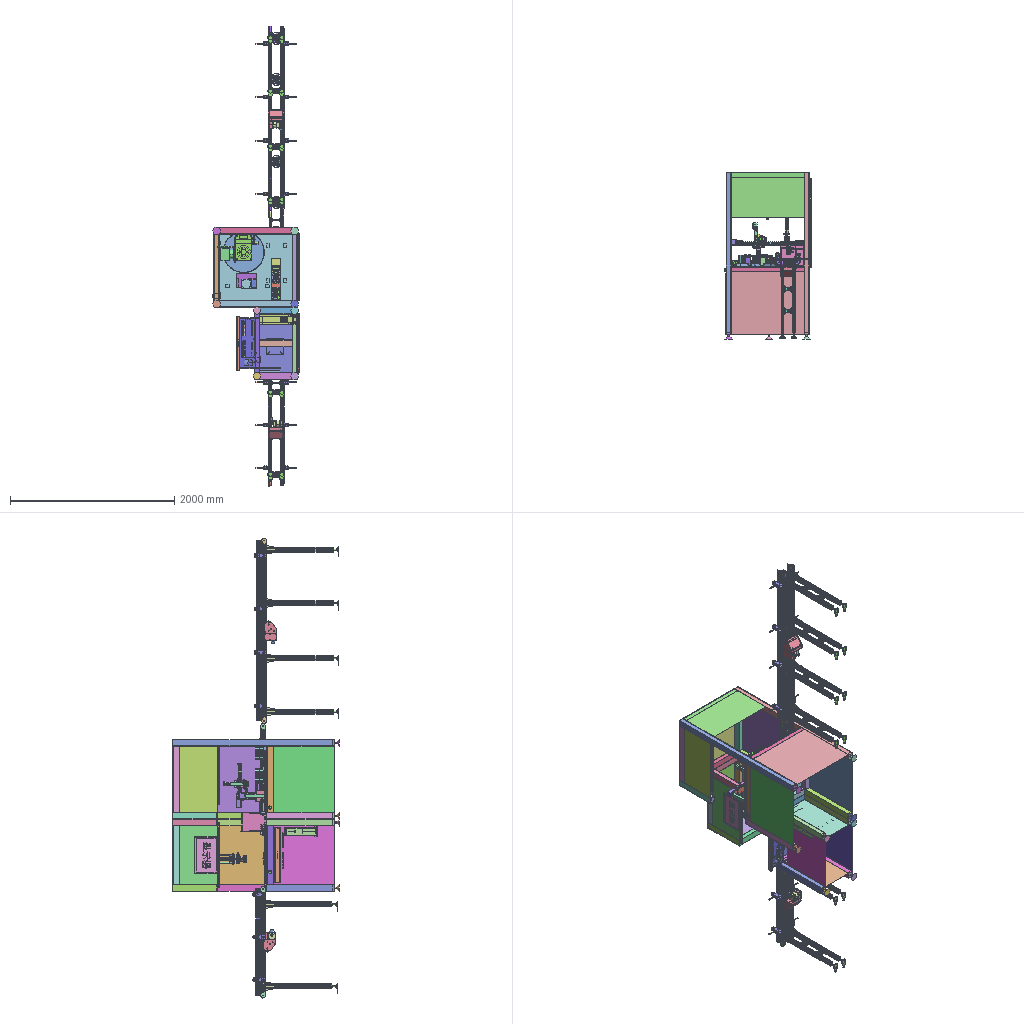Assembly | STEP file | 429 different items | 902 placed | box 1053 x 2031 x 5608 mm
Parts list (item | name | quantity | parent item | size | volume), first 276 of 429 items:
1 | Guide wheel mechanism revised.sldasm-Part-1 (subassembly) | x1 | in 导轮机构Assembly 2 | 80 x 1970 x 60 mm | 1583880 mm3
2 | Guide wheel mechanism revised.sldasm-Part-10 (subassembly) | x1 | in 导轮机构Assembly 2 | 80 x 60 x 890 mm | 715560 mm3
3 | Guide wheel mechanism revised.sldasm-Part-11 (subassembly) | x1 | in 导轮机构Assembly 2 | 972.42 x 1.2 x 1012 mm | 1181397 mm3
4 | Guide wheel mechanism revised.sldasm-Part-12 (subassembly) | x1 | in 导轮机构Assembly 2 | 91.505 x 80 x 91.505 mm | 172572 mm3
5 | Guide wheel mechanism revised.sldasm-Part-13 (subassembly) | x1 | in 导轮机构Assembly 2 | 91.505 x 80 x 91.505 mm | 172572 mm3
6 | Guide wheel mechanism revised.sldasm-Part-14 (subassembly) | x1 | in 导轮机构Assembly 2 | 91.505 x 80 x 91.505 mm | 172572 mm3
7 | Guide wheel mechanism revised.sldasm-Part-145 (subassembly) | x1 | in 导轮机构Assembly 2 | 80 x 1970 x 60 mm | 1583880 mm3
8 | Guide wheel mechanism revised.sldasm-Part-146 (subassembly) | x1 | in 导轮机构Assembly 2 | 80 x 1970 x 60 mm | 1583880 mm3
9 | Guide wheel mechanism revised.sldasm-Part-147 (subassembly) | x1 | in 导轮机构Assembly 2 | 720 x 80 x 60 mm | 578880 mm3
10 | Guide wheel mechanism revised.sldasm-Part-148 (subassembly) | x1 | in 导轮机构Assembly 2 | 720 x 80 x 60 mm | 578880 mm3
11 | Guide wheel mechanism revised.sldasm-Part-149 (subassembly) | x1 | in 导轮机构Assembly 2 | 720 x 80 x 60 mm | 578880 mm3
12 | Guide wheel mechanism revised.sldasm-Part-15 (subassembly) | x1 | in 导轮机构Assembly 2 | 91.505 x 80 x 91.505 mm | 172572 mm3
13 | Guide wheel mechanism revised.sldasm-Part-150 (subassembly) | x1 | in 导轮机构Assembly 2 | 720 x 80 x 60 mm | 578880 mm3
14 | Guide wheel mechanism revised.sldasm-Part-151 (subassembly) | x1 | in 导轮机构Assembly 2 | 80 x 60 x 400 mm | 321600 mm3
15 | Guide wheel mechanism revised.sldasm-Part-152 (subassembly) | x1 | in 导轮机构Assembly 2 | 80 x 60 x 400 mm | 321600 mm3
16 | Guide wheel mechanism revised.sldasm-Part-153 (subassembly) | x1 | in 导轮机构Assembly 2 | 80 x 60 x 400 mm | 321600 mm3
17 | Guide wheel mechanism revised.sldasm-Part-154 (subassembly) | x1 | in 导轮机构Assembly 2 | 80 x 60 x 400 mm | 321600 mm3
18 | Guide wheel mechanism revised.sldasm-Part-155 (subassembly) | x1 | in 导轮机构Assembly 2 | 80 x 60 x 400 mm | 321600 mm3
19 | Guide wheel mechanism revised.sldasm-Part-156 (subassembly) | x1 | in 导轮机构Assembly 2 | 80 x 60 x 400 mm | 321600 mm3
20 | Guide wheel mechanism revised.sldasm-Part-157 (subassembly) | x1 | in 导轮机构Assembly 2 | 882.42 x 8 x 522.42 mm | 3528427 mm3
21 | Guide wheel mechanism revised.sldasm-Part-158 (subassembly) | x1 | in 导轮机构Assembly 2 | 882.42 x 1.2 x 522.42 mm | 553193 mm3
22 | Guide wheel mechanism revised.sldasm-Part-159 (subassembly) | x1 | in 导轮机构Assembly 2 | 91.505 x 80 x 91.505 mm | 172572 mm3
23 | Guide wheel mechanism revised.sldasm-Part-16 (subassembly) | x1 | in 导轮机构Assembly 2 | 25 x 1120 x 25 mm | 195019 mm3
24 | Guide wheel mechanism revised.sldasm-Part-160 (subassembly) | x1 | in 导轮机构Assembly 2 | 91.505 x 80 x 91.505 mm | 172572 mm3
25 | Guide wheel mechanism revised.sldasm-Part-161 (subassembly) | x1 | in 导轮机构Assembly 2 | 91.505 x 80 x 91.505 mm | 172572 mm3
26 | Guide wheel mechanism revised.sldasm-Part-162 (subassembly) | x1 | in 导轮机构Assembly 2 | 91.505 x 80 x 91.505 mm | 172572 mm3
27 | Guide wheel mechanism revised.sldasm-Part-163 (subassembly) | x1 | in 导轮机构Assembly 2 | 25 x 1120 x 25 mm | 195019 mm3
28 | Guide wheel mechanism revised.sldasm-Part-164 (subassembly) | x1 | in 导轮机构Assembly 2 | 770 x 25 x 25 mm | 132103 mm3
29 | Guide wheel mechanism revised.sldasm-Part-165 (subassembly) | x1 | in 导轮机构Assembly 2 | 25 x 1120 x 25 mm | 195019 mm3
30 | Guide wheel mechanism revised.sldasm-Part-166 (subassembly) | x1 | in 导轮机构Assembly 2 | 770 x 25 x 25 mm | 132103 mm3
31 | Guide wheel mechanism revised.sldasm-Part-167 (subassembly) | x1 | in 导轮机构Assembly 2 | 720 x 740 x 2 mm | 886350 mm3
32 | Guide wheel mechanism revised.sldasm-Part-168 (subassembly) | x1 | in 导轮机构Assembly 2 | 1.2 x 760 x 400 mm | 364800 mm3
33 | Guide wheel mechanism revised.sldasm-Part-169 (subassembly) | x1 | in 导轮机构Assembly 2 | 2 x 760 x 403.01 mm | 612575 mm3
34 | Guide wheel mechanism revised.sldasm-Part-17 (subassembly) | x1 | in 导轮机构Assembly 2 | 860 x 25 x 25 mm | 148281 mm3
35 | Guide wheel mechanism revised.sldasm-Part-170 (subassembly) | x1 | in 导轮机构Assembly 2 | 720 x 740 x 1.2 mm | 639360 mm3
36 | Guide wheel mechanism revised.sldasm-Part-171 (subassembly) | x1 | in 导轮机构Assembly 2 | 80 x 828.01 x 60 mm | 665720 mm3
37 | Guide wheel mechanism revised.sldasm-Part-172 (subassembly) | x1 | in 导轮机构Assembly 2 | 80 x 541.99 x 60 mm | 435760 mm3
38 | Guide wheel mechanism revised.sldasm-Part-173 (subassembly) | x1 | in 导轮机构Assembly 2 | 74 x 5 x 54 mm | 19980 mm3
39 | Guide wheel mechanism revised.sldasm-Part-174 (subassembly) | x1 | in 导轮机构Assembly 2 | 74 x 5 x 54 mm | 19980 mm3
40 | Guide wheel mechanism revised.sldasm-Part-175 (subassembly) | x1 | in 导轮机构Assembly 2 | 80 x 60 x 400 mm | 321600 mm3
41 | Guide wheel mechanism revised.sldasm-Part-176 (subassembly) | x1 | in 导轮机构Assembly 2 | 80 x 60 x 400 mm | 217600 mm3
42 | Guide wheel mechanism revised.sldasm-Part-177 (subassembly) | x1 | in 导轮机构Assembly 2 | 720 x 60 x 80 mm | 578880 mm3
43 | Guide wheel mechanism revised.sldasm-Part-178 (subassembly) | x1 | in 导轮机构Assembly 2 | 80 x 828.01 x 60 mm | 665720 mm3
44 | Guide wheel mechanism revised.sldasm-Part-179 (subassembly) | x1 | in 导轮机构Assembly 2 | 80 x 541.99 x 60 mm | 435760 mm3
45 | Guide wheel mechanism revised.sldasm-Part-18 (subassembly) | x1 | in 导轮机构Assembly 2 | 25 x 1120 x 25 mm | 195019 mm3
46 | Guide wheel mechanism revised.sldasm-Part-180 (subassembly) | x1 | in 导轮机构Assembly 2 | 74 x 5 x 54 mm | 19980 mm3
47 | Guide wheel mechanism revised.sldasm-Part-181 (subassembly) | x1 | in 导轮机构Assembly 2 | 74 x 5 x 54 mm | 19980 mm3
48 | Guide wheel mechanism revised.sldasm-Part-182 (subassembly) | x1 | in 导轮机构Assembly 2 | 735 x 1085 x 1.2 mm | 956970 mm3
49 | Guide wheel mechanism revised.sldasm-Part-183 (subassembly) | x1 | in 导轮机构Assembly 2 | 5 x 421.99 x 400 mm | 843980 mm3
50 | Guide wheel mechanism revised.sldasm-Part-184 (subassembly) | x1 | in 导轮机构Assembly 2 | 720 x 461.99 x 3 mm | 633248 mm3
51 | Guide wheel mechanism revised.sldasm-Part-185 (subassembly) | x1 | in 导轮机构Assembly 2 | 22.5 x 75 x 250 mm | 43875 mm3
52 | Guide wheel mechanism revised.sldasm-Part-186 (subassembly) | x1 | in 导轮机构Assembly 2 | 22.5 x 75 x 250 mm | 43875 mm3
53 | Guide wheel mechanism revised.sldasm-Part-187 (subassembly) | x1 | in 导轮机构Assembly 2 | 123 x 31.5 x 458.8 mm | 125941 mm3
54 | Guide wheel mechanism revised.sldasm-Part-188 (subassembly) | x1 | in 导轮机构Assembly 2 | 38 x 275 x 47 mm | 67650 mm3
55 | Guide wheel mechanism revised.sldasm-Part-189 (subassembly) | x1 | in 导轮机构Assembly 2 | 38 x 275 x 45.79 mm | 66652 mm3
56 | Guide wheel mechanism revised.sldasm-Part-19 (subassembly) | x1 | in 导轮机构Assembly 2 | 860 x 25 x 25 mm | 148281 mm3
57 | Guide wheel mechanism revised.sldasm-Part-190 (subassembly) | x1 | in 导轮机构Assembly 2 | 660 x 50 x 30 mm | 98910 mm3
58 | Guide wheel mechanism revised.sldasm-Part-191 (subassembly) | x1 | in 导轮机构Assembly 2 | 600 x 35 x 200 mm | 241391 mm3
59 | Guide wheel mechanism revised.sldasm-Part-192 (subassembly) | x1 | in 导轮机构Assembly 2 | 420.5 x 396 x 106 mm | 15546252 mm3
60 | Guide wheel mechanism revised.sldasm-Part-193 (subassembly) | x2 | in 导轮机构Assembly 2 | 505 x 45 x 12.5 mm | 214790 mm3
61 | Guide wheel mechanism revised.sldasm-Part-194 (subassembly) | x1 | in 导轮机构Assembly 2 | 93.5 x 80 x 103 mm | 26904 mm3
62 | Guide wheel mechanism revised.sldasm-Part-195 (subassembly) | x1 | in 导轮机构Assembly 2 | - | -
63 | Guide wheel mechanism revised.sldasm-Part-196 (subassembly) | x1 | in 导轮机构Assembly 2 | - | -
64 | Guide wheel mechanism revised.sldasm-Part-197 (subassembly) | x1 | in 导轮机构Assembly 2 | - | -
65 | Guide wheel mechanism revised.sldasm-Part-198 (subassembly) | x1 | in 导轮机构Assembly 2 | - | -
66 | Guide wheel mechanism revised.sldasm-Part-199 (subassembly) | x1 | in 导轮机构Assembly 2 | - | -
67 | Guide wheel mechanism revised.sldasm-Part-2 (subassembly) | x1 | in 导轮机构Assembly 2 | 80 x 1970 x 60 mm | 1583880 mm3
68 | Guide wheel mechanism revised.sldasm-Part-20 (subassembly) | x1 | in 导轮机构Assembly 2 | 825 x 1085 x 2 mm | 1790250 mm3
69 | Guide wheel mechanism revised.sldasm-Part-200 (subassembly) | x1 | in 导轮机构Assembly 2 | - | -
70 | Guide wheel mechanism revised.sldasm-Part-201 (subassembly) | x1 | in 导轮机构Assembly 2 | - | -
71 | Guide wheel mechanism revised.sldasm-Part-202 (subassembly) | x1 | in 导轮机构Assembly 2 | - | -
72 | Guide wheel mechanism revised.sldasm-Part-203 (subassembly) | x1 | in 导轮机构Assembly 2 | - | -
73 | Guide wheel mechanism revised.sldasm-Part-204 (subassembly) | x1 | in 导轮机构Assembly 2 | - | -
74 | Guide wheel mechanism revised.sldasm-Part-205 (subassembly) | x1 | in 导轮机构Assembly 2 | - | -
75 | Guide wheel mechanism revised.sldasm-Part-206 (subassembly) | x1 | in 导轮机构Assembly 2 | - | -
76 | Guide wheel mechanism revised.sldasm-Part-207 (subassembly) | x1 | in 导轮机构Assembly 2 | - | -
77 | Guide wheel mechanism revised.sldasm-Part-208 (subassembly) | x1 | in 导轮机构Assembly 2 | - | -
78 | Guide wheel mechanism revised.sldasm-Part-209 (subassembly) | x1 | in 导轮机构Assembly 2 | - | -
79 | Guide wheel mechanism revised.sldasm-Part-21 (subassembly) | x1 | in 导轮机构Assembly 2 | 810 x 740 x 5 mm | 2997000 mm3
80 | Guide wheel mechanism revised.sldasm-Part-210 (subassembly) | x1 | in 导轮机构Assembly 2 | - | -
81 | Guide wheel mechanism revised.sldasm-Part-211 (subassembly) | x1 | in 导轮机构Assembly 2 | - | -
82 | Guide wheel mechanism revised.sldasm-Part-212 (subassembly) | x1 | in 导轮机构Assembly 2 | - | -
83 | Guide wheel mechanism revised.sldasm-Part-213 (subassembly) | x1 | in 导轮机构Assembly 2 | - | -
84 | Guide wheel mechanism revised.sldasm-Part-214 (subassembly) | x1 | in 导轮机构Assembly 2 | - | -
85 | Guide wheel mechanism revised.sldasm-Part-215 (subassembly) | x1 | in 导轮机构Assembly 2 | - | -
86 | Guide wheel mechanism revised.sldasm-Part-216 (subassembly) | x1 | in 导轮机构Assembly 2 | - | -
87 | Guide wheel mechanism revised.sldasm-Part-217 (subassembly) | x1 | in 导轮机构Assembly 2 | - | -
88 | Guide wheel mechanism revised.sldasm-Part-218 (subassembly) | x1 | in 导轮机构Assembly 2 | - | -
89 | Guide wheel mechanism revised.sldasm-Part-219 (subassembly) | x1 | in 导轮机构Assembly 2 | - | -
90 | Guide wheel mechanism revised.sldasm-Part-22 (subassembly) | x1 | in 导轮机构Assembly 2 | 1.2 x 760 x 890 mm | 811680 mm3
91 | Guide wheel mechanism revised.sldasm-Part-220 (subassembly) | x1 | in 导轮机构Assembly 2 | - | -
92 | Guide wheel mechanism revised.sldasm-Part-221 (subassembly) | x1 | in 导轮机构Assembly 2 | - | -
93 | Guide wheel mechanism revised.sldasm-Part-222 (subassembly) | x1 | in 导轮机构Assembly 2 | - | -
94 | Guide wheel mechanism revised.sldasm-Part-223 (subassembly) | x1 | in 导轮机构Assembly 2 | - | -
95 | Guide wheel mechanism revised.sldasm-Part-224 (subassembly) | x1 | in 导轮机构Assembly 2 | - | -
96 | Guide wheel mechanism revised.sldasm-Part-225 (subassembly) | x1 | in 导轮机构Assembly 2 | - | -
97 | Guide wheel mechanism revised.sldasm-Part-226 (subassembly) | x1 | in 导轮机构Assembly 2 | - | -
98 | Guide wheel mechanism revised.sldasm-Part-227 (subassembly) | x1 | in 导轮机构Assembly 2 | - | -
99 | Guide wheel mechanism revised.sldasm-Part-228 (subassembly) | x1 | in 导轮机构Assembly 2 | - | -
100 | Guide wheel mechanism revised.sldasm-Part-229 (subassembly) | x1 | in 导轮机构Assembly 2 | - | -
101 | Guide wheel mechanism revised.sldasm-Part-23 (subassembly) | x1 | in 导轮机构Assembly 2 | 810 x 740 x 5 mm | 2997000 mm3
102 | Guide wheel mechanism revised.sldasm-Part-230 (subassembly) | x1 | in 导轮机构Assembly 2 | - | -
103 | Guide wheel mechanism revised.sldasm-Part-231 (subassembly) | x1 | in 导轮机构Assembly 2 | - | -
104 | Guide wheel mechanism revised.sldasm-Part-232 (subassembly) | x1 | in 导轮机构Assembly 2 | - | -
105 | Guide wheel mechanism revised.sldasm-Part-233 (subassembly) | x1 | in 导轮机构Assembly 2 | - | -
106 | Guide wheel mechanism revised.sldasm-Part-234 (subassembly) | x1 | in 导轮机构Assembly 2 | - | -
107 | Guide wheel mechanism revised.sldasm-Part-235 (subassembly) | x1 | in 导轮机构Assembly 2 | - | -
108 | Guide wheel mechanism revised.sldasm-Part-236 (subassembly) | x1 | in 导轮机构Assembly 2 | - | -
109 | Guide wheel mechanism revised.sldasm-Part-237 (subassembly) | x1 | in 导轮机构Assembly 2 | - | -
110 | Guide wheel mechanism revised.sldasm-Part-238 (subassembly) | x1 | in 导轮机构Assembly 2 | - | -
111 | Guide wheel mechanism revised.sldasm-Part-239 (subassembly) | x1 | in 导轮机构Assembly 2 | - | -
112 | Guide wheel mechanism revised.sldasm-Part-24 (subassembly) | x1 | in 导轮机构Assembly 2 | 810 x 461.99 x 1.2 mm | 449054 mm3
113 | Guide wheel mechanism revised.sldasm-Part-240 (subassembly) | x1 | in 导轮机构Assembly 2 | - | -
114 | Guide wheel mechanism revised.sldasm-Part-241 (subassembly) | x1 | in 导轮机构Assembly 2 | - | -
115 | Guide wheel mechanism revised.sldasm-Part-242 (subassembly) | x1 | in 导轮机构Assembly 2 | - | -
116 | Guide wheel mechanism revised.sldasm-Part-243 (subassembly) | x1 | in 导轮机构Assembly 2 | - | -
117 | Guide wheel mechanism revised.sldasm-Part-244 (subassembly) | x1 | in 导轮机构Assembly 2 | - | -
118 | Guide wheel mechanism revised.sldasm-Part-245 (subassembly) | x1 | in 导轮机构Assembly 2 | - | -
119 | Guide wheel mechanism revised.sldasm-Part-246 (subassembly) | x1 | in 导轮机构Assembly 2 | - | -
120 | Guide wheel mechanism revised.sldasm-Part-247 (subassembly) | x1 | in 导轮机构Assembly 2 | - | -
121 | Guide wheel mechanism revised.sldasm-Part-248 (subassembly) | x1 | in 导轮机构Assembly 2 | - | -
122 | Guide wheel mechanism revised.sldasm-Part-249 (subassembly) | x1 | in 导轮机构Assembly 2 | - | -
123 | Guide wheel mechanism revised.sldasm-Part-25 (subassembly) | x1 | in 导轮机构Assembly 2 | 80 x 828.01 x 60 mm | 665720 mm3
124 | Guide wheel mechanism revised.sldasm-Part-250 (subassembly) | x1 | in 导轮机构Assembly 2 | - | -
125 | Guide wheel mechanism revised.sldasm-Part-251 (subassembly) | x1 | in 导轮机构Assembly 2 | - | -
126 | Guide wheel mechanism revised.sldasm-Part-252 (subassembly) | x1 | in 导轮机构Assembly 2 | - | -
127 | Guide wheel mechanism revised.sldasm-Part-253 (subassembly) | x1 | in 导轮机构Assembly 2 | - | -
128 | Guide wheel mechanism revised.sldasm-Part-254 (subassembly) | x1 | in 导轮机构Assembly 2 | - | -
129 | Guide wheel mechanism revised.sldasm-Part-255 (subassembly) | x1 | in 导轮机构Assembly 2 | - | -
130 | Guide wheel mechanism revised.sldasm-Part-256 (subassembly) | x1 | in 导轮机构Assembly 2 | - | -
131 | Guide wheel mechanism revised.sldasm-Part-257 (subassembly) | x1 | in 导轮机构Assembly 2 | - | -
132 | Guide wheel mechanism revised.sldasm-Part-258 (subassembly) | x1 | in 导轮机构Assembly 2 | - | -
133 | Guide wheel mechanism revised.sldasm-Part-259 (subassembly) | x1 | in 导轮机构Assembly 2 | - | -
134 | Guide wheel mechanism revised.sldasm-Part-26 (subassembly) | x1 | in 导轮机构Assembly 2 | 80 x 541.99 x 60 mm | 435760 mm3
135 | Guide wheel mechanism revised.sldasm-Part-260 (subassembly) | x1 | in 导轮机构Assembly 2 | - | -
136 | Guide wheel mechanism revised.sldasm-Part-261 (subassembly) | x1 | in 导轮机构Assembly 2 | - | -
137 | Guide wheel mechanism revised.sldasm-Part-262 (subassembly) | x1 | in 导轮机构Assembly 2 | - | -
138 | Guide wheel mechanism revised.sldasm-Part-263 (subassembly) | x1 | in 导轮机构Assembly 2 | - | -
139 | Guide wheel mechanism revised.sldasm-Part-264 (subassembly) | x1 | in 导轮机构Assembly 2 | - | -
140 | Guide wheel mechanism revised.sldasm-Part-265 (subassembly) | x1 | in 导轮机构Assembly 2 | - | -
141 | Guide wheel mechanism revised.sldasm-Part-266 (subassembly) | x1 | in 导轮机构Assembly 2 | - | -
142 | Guide wheel mechanism revised.sldasm-Part-267 (subassembly) | x1 | in 导轮机构Assembly 2 | - | -
143 | Guide wheel mechanism revised.sldasm-Part-268 (subassembly) | x1 | in 导轮机构Assembly 2 | - | -
144 | Guide wheel mechanism revised.sldasm-Part-269 (subassembly) | x1 | in 导轮机构Assembly 2 | - | -
145 | Guide wheel mechanism revised.sldasm-Part-27 (subassembly) | x1 | in 导轮机构Assembly 2 | 74 x 5 x 54 mm | 19980 mm3
146 | Guide wheel mechanism revised.sldasm-Part-270 (subassembly) | x1 | in 导轮机构Assembly 2 | - | -
147 | Guide wheel mechanism revised.sldasm-Part-271 (subassembly) | x1 | in 导轮机构Assembly 2 | - | -
148 | Guide wheel mechanism revised.sldasm-Part-272 (subassembly) | x1 | in 导轮机构Assembly 2 | - | -
149 | Guide wheel mechanism revised.sldasm-Part-273 (subassembly) | x1 | in 导轮机构Assembly 2 | - | -
150 | Guide wheel mechanism revised.sldasm-Part-274 (subassembly) | x1 | in 导轮机构Assembly 2 | - | -
151 | Guide wheel mechanism revised.sldasm-Part-275 (subassembly) | x1 | in 导轮机构Assembly 2 | - | -
152 | Guide wheel mechanism revised.sldasm-Part-276 (subassembly) | x1 | in 导轮机构Assembly 2 | - | -
153 | Guide wheel mechanism revised.sldasm-Part-277 (subassembly) | x1 | in 导轮机构Assembly 2 | - | -
154 | Guide wheel mechanism revised.sldasm-Part-278 (subassembly) | x1 | in 导轮机构Assembly 2 | - | -
155 | Guide wheel mechanism revised.sldasm-Part-279 (subassembly) | x1 | in 导轮机构Assembly 2 | - | -
156 | Guide wheel mechanism revised.sldasm-Part-28 (subassembly) | x1 | in 导轮机构Assembly 2 | 74 x 5 x 54 mm | 19980 mm3
157 | Guide wheel mechanism revised.sldasm-Part-280 (subassembly) | x1 | in 导轮机构Assembly 2 | - | -
158 | Guide wheel mechanism revised.sldasm-Part-281 (subassembly) | x1 | in 导轮机构Assembly 2 | - | -
159 | Guide wheel mechanism revised.sldasm-Part-282 (subassembly) | x1 | in 导轮机构Assembly 2 | - | -
160 | Guide wheel mechanism revised.sldasm-Part-283 (subassembly) | x1 | in 导轮机构Assembly 2 | - | -
161 | Guide wheel mechanism revised.sldasm-Part-284 (subassembly) | x1 | in 导轮机构Assembly 2 | - | -
162 | Guide wheel mechanism revised.sldasm-Part-285 (subassembly) | x1 | in 导轮机构Assembly 2 | - | -
163 | Guide wheel mechanism revised.sldasm-Part-286 (subassembly) | x1 | in 导轮机构Assembly 2 | - | -
164 | Guide wheel mechanism revised.sldasm-Part-287 (subassembly) | x1 | in 导轮机构Assembly 2 | - | -
165 | Guide wheel mechanism revised.sldasm-Part-288 (subassembly) | x1 | in 导轮机构Assembly 2 | - | -
166 | Guide wheel mechanism revised.sldasm-Part-289 (subassembly) | x1 | in 导轮机构Assembly 2 | - | -
167 | Guide wheel mechanism revised.sldasm-Part-29 (subassembly) | x1 | in 导轮机构Assembly 2 | 1.2 x 481.99 x 890 mm | 514765 mm3
168 | Guide wheel mechanism revised.sldasm-Part-290 (subassembly) | x1 | in 导轮机构Assembly 2 | - | -
169 | Guide wheel mechanism revised.sldasm-Part-291 (subassembly) | x1 | in 导轮机构Assembly 2 | - | -
170 | Guide wheel mechanism revised.sldasm-Part-292 (subassembly) | x1 | in 导轮机构Assembly 2 | - | -
171 | Guide wheel mechanism revised.sldasm-Part-293 (subassembly) | x1 | in 导轮机构Assembly 2 | - | -
172 | Guide wheel mechanism revised.sldasm-Part-294 (subassembly) | x1 | in 导轮机构Assembly 2 | - | -
173 | Guide wheel mechanism revised.sldasm-Part-295 (subassembly) | x1 | in 导轮机构Assembly 2 | - | -
174 | Guide wheel mechanism revised.sldasm-Part-296 (subassembly) | x1 | in 导轮机构Assembly 2 | - | -
175 | Guide wheel mechanism revised.sldasm-Part-297 (subassembly) | x1 | in 导轮机构Assembly 2 | - | -
176 | Guide wheel mechanism revised.sldasm-Part-298 (subassembly) | x1 | in 导轮机构Assembly 2 | - | -
177 | Guide wheel mechanism revised.sldasm-Part-299 (subassembly) | x1 | in 导轮机构Assembly 2 | - | -
178 | Guide wheel mechanism revised.sldasm-Part-3 (subassembly) | x1 | in 导轮机构Assembly 2 | 80 x 1970 x 60 mm | 1583880 mm3
179 | Guide wheel mechanism revised.sldasm-Part-30 (subassembly) | x1 | in 导轮机构Assembly 2 | 80 x 60 x 890 mm | 705411 mm3
180 | Guide wheel mechanism revised.sldasm-Part-300 (subassembly) | x1 | in 导轮机构Assembly 2 | - | -
181 | Guide wheel mechanism revised.sldasm-Part-301 (subassembly) | x1 | in 导轮机构Assembly 2 | - | -
182 | Guide wheel mechanism revised.sldasm-Part-302 (subassembly) | x1 | in 导轮机构Assembly 2 | - | -
183 | Guide wheel mechanism revised.sldasm-Part-303 (subassembly) | x1 | in 导轮机构Assembly 2 | - | -
184 | Guide wheel mechanism revised.sldasm-Part-304 (subassembly) | x1 | in 导轮机构Assembly 2 | - | -
185 | Guide wheel mechanism revised.sldasm-Part-305 (subassembly) | x1 | in 导轮机构Assembly 2 | - | -
186 | Guide wheel mechanism revised.sldasm-Part-306 (subassembly) | x1 | in 导轮机构Assembly 2 | - | -
187 | Guide wheel mechanism revised.sldasm-Part-307 (subassembly) | x1 | in 导轮机构Assembly 2 | - | 200.153 mm3
188 | Guide wheel mechanism revised.sldasm-Part-308 (subassembly) | x1 | in 导轮机构Assembly 2 | 37.055 x 16.939 x 57.91 mm | 1764 mm3
189 | Guide wheel mechanism revised.sldasm-Part-309 (subassembly) | x1 | in 导轮机构Assembly 2 | 37.025 x 17.101 x 57.898 mm | 1738 mm3
190 | Guide wheel mechanism revised.sldasm-Part-31 (subassembly) | x1 | in 导轮机构Assembly 2 | 972.42 x 8 x 1012 mm | 5346860 mm3
191 | Guide wheel mechanism revised.sldasm-Part-310 (subassembly) | x1 | in 导轮机构Assembly 2 | 8 x 21.346 x 21.346 mm | 2417 mm3
192 | Guide wheel mechanism revised.sldasm-Part-311 (subassembly) | x1 | in 导轮机构Assembly 2 | 231.61 x 29.722 x 176.987 mm | 19601 mm3
193 | Guide wheel mechanism revised.sldasm-Part-312 (subassembly) | x1 | in 导轮机构Assembly 2 | 95 x 70 x 25 mm | 34478 mm3
194 | Guide wheel mechanism revised.sldasm-Part-313 (subassembly) | x1 | in 导轮机构Assembly 2 | 440 x 275 x 55 mm | 5174621 mm3
195 | Guide wheel mechanism revised.sldasm-Part-314 (subassembly) | x1 | in 导轮机构Assembly 2 | 520 x 120 x 10 mm | 105158 mm3
196 | Guide wheel mechanism revised.sldasm-Part-315 (subassembly) | x2 | in 导轮机构Assembly 2 | 28 x 790 x 26.2 mm | 498619 mm3
197 | Guide wheel mechanism revised.sldasm-Part-316 (subassembly) | x2 | in 导轮机构Assembly 2 | 8.3 x 36.4 x 10.5 mm | 2626 mm3
198 | Guide wheel mechanism revised.sldasm-Part-317 (subassembly) | x2 | in 导轮机构Assembly 2 | 8.3 x 36.4 x 40.2 mm | 3466 mm3
199 | Guide wheel mechanism revised.sldasm-Part-318 (subassembly) | x1 | in 导轮机构Assembly 2 | 88 x 37 x 88 mm | 180795 mm3
200 | Guide wheel mechanism revised.sldasm-Part-319 (subassembly) | x1 | in 导轮机构Assembly 2 | 200 x 10 x 200 mm | 395602 mm3
201 | Guide wheel mechanism revised.sldasm-Part-32 (subassembly) | x2 | in 导轮机构Assembly 2 | 28 x 710 x 26.2 mm | 446680 mm3
202 | Guide wheel mechanism revised.sldasm-Part-320 (subassembly) | x8 | in 导轮机构Assembly 2 | 16 x 30 x 16 mm | 2413 mm3
203 | Guide wheel mechanism revised.sldasm-Part-321 (subassembly) | x1 | in 导轮机构Assembly 2 | - | -
204 | Guide wheel mechanism revised.sldasm-Part-322 (subassembly) | x1 | in 导轮机构Assembly 2 | - | -
205 | Guide wheel mechanism revised.sldasm-Part-323 (subassembly) | x1 | in 导轮机构Assembly 2 | - | -
206 | Guide wheel mechanism revised.sldasm-Part-324 (subassembly) | x1 | in 导轮机构Assembly 2 | - | -
207 | Guide wheel mechanism revised.sldasm-Part-325 (subassembly) | x1 | in 导轮机构Assembly 2 | - | -
208 | Guide wheel mechanism revised.sldasm-Part-326 (subassembly) | x1 | in 导轮机构Assembly 2 | - | -
209 | Guide wheel mechanism revised.sldasm-Part-327 (subassembly) | x1 | in 导轮机构Assembly 2 | 1360 x 54 x 186 mm | 2730311 mm3
210 | Guide wheel mechanism revised.sldasm-Part-328 (subassembly) | x2 | in 导轮机构Assembly 2 | 1359 x 59 x 20 mm | 249410 mm3
211 | Guide wheel mechanism revised.sldasm-Part-329 (subassembly) | x2 | in 导轮机构Assembly 2 | 14 x 50 x 1300 mm | 330720 mm3
212 | Guide wheel mechanism revised.sldasm-Part-33 (subassembly) | x2 | in 导轮机构Assembly 2 | 8.3 x 36.4 x 10.5 mm | 2626 mm3
213 | Guide wheel mechanism revised.sldasm-Part-330 (subassembly) | x2 | in 导轮机构Assembly 2 | 12 x 56 x 1300 mm | 319800 mm3
214 | Guide wheel mechanism revised.sldasm-Part-331 (subassembly) | x1 | in 导轮机构Assembly 2 | 303.8 x 300 x 230 mm | 338755 mm3
215 | Guide wheel mechanism revised.sldasm-Part-332 (subassembly) | x2 | in 导轮机构Assembly 2 | 5.4 x 300 x 6.2 mm | 5131 mm3
216 | Guide wheel mechanism revised.sldasm-Part-333 (subassembly) | x1 | in 导轮机构Assembly 2 | 282 x 320 x 2.5 mm | 102141 mm3
217 | Guide wheel mechanism revised.sldasm-Part-334 (subassembly) | x2 | in 导轮机构Assembly 2 | 75 x 65 x 75 mm | 65636 mm3
218 | Guide wheel mechanism revised.sldasm-Part-335 (subassembly) | x2 | in 导轮机构Assembly 2 | 60 x 85 x 60 mm | 60625 mm3
219 | Guide wheel mechanism revised.sldasm-Part-336 (subassembly) | x6 | in 导轮机构Assembly 2 | 40 x 105 x 40 mm | 36538 mm3
220 | Guide wheel mechanism revised.sldasm-Part-337 (subassembly) | x1 | in 导轮机构Assembly 2 | 500 x 50 x 500 mm | 2751729 mm3
221 | Guide wheel mechanism revised.sldasm-Part-338 (subassembly) | x1 | in 导轮机构Assembly 2 | - | -
222 | Guide wheel mechanism revised.sldasm-Part-339 (subassembly) | x1 | in 导轮机构Assembly 2 | - | -
223 | Guide wheel mechanism revised.sldasm-Part-34 (subassembly) | x2 | in 导轮机构Assembly 2 | 8.3 x 36.4 x 40.2 mm | 3466 mm3
224 | Guide wheel mechanism revised.sldasm-Part-343 (subassembly) | x1 | in 导轮机构Assembly 2 | - | -
225 | Guide wheel mechanism revised.sldasm-Part-344 (subassembly) | x1 | in 导轮机构Assembly 2 | - | -
226 | Guide wheel mechanism revised.sldasm-Part-345 (subassembly) | x1 | in 导轮机构Assembly 2 | - | -
227 | Guide wheel mechanism revised.sldasm-Part-346 (subassembly) | x1 | in 导轮机构Assembly 2 | - | -
228 | Guide wheel mechanism revised.sldasm-Part-347 (subassembly) | x1 | in 导轮机构Assembly 2 | - | -
229 | Guide wheel mechanism revised.sldasm-Part-348 (subassembly) | x6 | in 导轮机构Assembly 2 | 100 x 10 x 100 mm | 48975 mm3
230 | Guide wheel mechanism revised.sldasm-Part-349 (subassembly) | x1 | in 导轮机构Assembly 2 | 85 x 255 x 85 mm | 157022 mm3
231 | Guide wheel mechanism revised.sldasm-Part-35 (subassembly) | x2 | in 导轮机构Assembly 2 | 28 x 390 x 26.2 mm | 238924 mm3
232 | Guide wheel mechanism revised.sldasm-Part-350 (subassembly) | x1 | in 导轮机构Assembly 2 | 52 x 50 x 34 mm | 44573 mm3
233 | Guide wheel mechanism revised.sldasm-Part-351 (subassembly) | x1 | in 导轮机构Assembly 2 | 270 x 15 x 15 mm | 45909 mm3
234 | Guide wheel mechanism revised.sldasm-Part-352 (subassembly) | x1 | in 导轮机构Assembly 2 | 5 x 21 x 21 mm | 1037 mm3
235 | Guide wheel mechanism revised.sldasm-Part-353 (subassembly) | x1 | in 导轮机构Assembly 2 | 5 x 19 x 19 mm | 911.062 mm3
236 | Guide wheel mechanism revised.sldasm-Part-354 (subassembly) | x1 | in 导轮机构Assembly 2 | 85 x 30 x 111 mm | 43979 mm3
237 | Guide wheel mechanism revised.sldasm-Part-355 (subassembly) | x1 | in 导轮机构Assembly 2 | 110 x 110 x 170 mm | 1274045 mm3
238 | Guide wheel mechanism revised.sldasm-Part-356 (subassembly) | x3 | in 导轮机构Assembly 2 | 32.2 x 28 x 28 mm | 14007 mm3
239 | Guide wheel mechanism revised.sldasm-Part-357 (subassembly) | x1 | in 导轮机构Assembly 2 | 175 x 5 x 250 mm | 216933 mm3
240 | Guide wheel mechanism revised.sldasm-Part-358 (subassembly) | x1 | in 导轮机构Assembly 2 | 60 x 74 x 5 mm | 11100 mm3
241 | Guide wheel mechanism revised.sldasm-Part-359 (subassembly) | x1 | in 导轮机构Assembly 2 | 60 x 74 x 5 mm | 11100 mm3
242 | Guide wheel mechanism revised.sldasm-Part-36 (subassembly) | x2 | in 导轮机构Assembly 2 | 8.3 x 36.4 x 10.5 mm | 2626 mm3
243 | Guide wheel mechanism revised.sldasm-Part-360 (subassembly) | x1 | in 导轮机构Assembly 2 | 180 x 79 x 110 mm | 133597 mm3
244 | Guide wheel mechanism revised.sldasm-Part-361 (subassembly) | x1 | in 导轮机构Assembly 2 | - | -
245 | Guide wheel mechanism revised.sldasm-Part-362 (subassembly) | x1 | in 导轮机构Assembly 2 | - | -
246 | Guide wheel mechanism revised.sldasm-Part-363 (subassembly) | x1 | in 导轮机构Assembly 2 | - | -
247 | Guide wheel mechanism revised.sldasm-Part-364 (subassembly) | x1 | in 导轮机构Assembly 2 | - | -
248 | Guide wheel mechanism revised.sldasm-Part-365 (subassembly) | x1 | in 导轮机构Assembly 2 | - | -
249 | Guide wheel mechanism revised.sldasm-Part-366 (subassembly) | x1 | in 导轮机构Assembly 2 | - | -
250 | Guide wheel mechanism revised.sldasm-Part-367 (subassembly) | x1 | in 导轮机构Assembly 2 | - | -
251 | Guide wheel mechanism revised.sldasm-Part-368 (subassembly) | x1 | in 导轮机构Assembly 2 | - | -
252 | Guide wheel mechanism revised.sldasm-Part-369 (subassembly) | x1 | in 导轮机构Assembly 2 | - | -
253 | Guide wheel mechanism revised.sldasm-Part-37 (subassembly) | x2 | in 导轮机构Assembly 2 | 8.3 x 36.4 x 40.2 mm | 3466 mm3
254 | Guide wheel mechanism revised.sldasm-Part-370 (subassembly) | x1 | in 导轮机构Assembly 2 | - | -
255 | Guide wheel mechanism revised.sldasm-Part-371 (subassembly) | x1 | in 导轮机构Assembly 2 | - | -
256 | Guide wheel mechanism revised.sldasm-Part-372 (subassembly) | x1 | in 导轮机构Assembly 2 | - | -
257 | Guide wheel mechanism revised.sldasm-Part-373 (subassembly) | x1 | in 导轮机构Assembly 2 | - | -
258 | Guide wheel mechanism revised.sldasm-Part-374 (subassembly) | x1 | in 导轮机构Assembly 2 | - | -
259 | Guide wheel mechanism revised.sldasm-Part-375 (subassembly) | x1 | in 导轮机构Assembly 2 | 50 x 14 x 54 mm | 10336 mm3
260 | Guide wheel mechanism revised.sldasm-Part-376 (subassembly) | x4 | in 导轮机构Assembly 2 | 12 x 7 x 7 mm | 237.501 mm3
261 | Guide wheel mechanism revised.sldasm-Part-377 (subassembly) | x1 | in 导轮机构Assembly 2 | 90 x 18.7 x 40 mm | 39818 mm3
262 | Guide wheel mechanism revised.sldasm-Part-378 (subassembly) | x1 | in 导轮机构Assembly 2 | 60 x 6 x 60 mm | 19638 mm3
263 | Guide wheel mechanism revised.sldasm-Part-379 (subassembly) | x1 | in 导轮机构Assembly 2 | 90 x 24.3 x 84.5 mm | 59688 mm3
264 | Guide wheel mechanism revised.sldasm-Part-38 (subassembly) | x1 | in 导轮机构Assembly 2 | 100 x 224 x 19.6 mm | 404407 mm3
265 | Guide wheel mechanism revised.sldasm-Part-380 (subassembly) | x1 | in 导轮机构Assembly 2 | 52.6 x 11.5 x 42.9 mm | 14076 mm3
266 | Guide wheel mechanism revised.sldasm-Part-381 (subassembly) | x1 | in 导轮机构Assembly 2 | 41.75 x 21.5 x 81.45 mm | 18105 mm3
267 | Guide wheel mechanism revised.sldasm-Part-382 (subassembly) | x1 | in 导轮机构Assembly 2 | 58.5 x 13 x 13 mm | 2266 mm3
268 | Guide wheel mechanism revised.sldasm-Part-383 (subassembly) | x3 | in 导轮机构Assembly 2 | 20 x 23 x 90 mm | 7697 mm3
269 | Guide wheel mechanism revised.sldasm-Part-384 (subassembly) | x3 | in 导轮机构Assembly 2 | - | -
270 | Guide wheel mechanism revised.sldasm-Part-385 (subassembly) | x3 | in 导轮机构Assembly 2 | - | -
271 | Guide wheel mechanism revised.sldasm-Part-386 (subassembly) | x3 | in 导轮机构Assembly 2 | - | -
272 | Guide wheel mechanism revised.sldasm-Part-387 (subassembly) | x3 | in 导轮机构Assembly 2 | - | -
273 | Guide wheel mechanism revised.sldasm-Part-388 (subassembly) | x3 | in 导轮机构Assembly 2 | - | -
274 | Guide wheel mechanism revised.sldasm-Part-389 (subassembly) | x3 | in 导轮机构Assembly 2 | - | -
275 | Guide wheel mechanism revised.sldasm-Part-39 (subassembly) | x2 | in 导轮机构Assembly 2 | 280 x 16 x 16 mm | 56107 mm3
276 | Guide wheel mechanism revised.sldasm-Part-390 (subassembly) | x3 | in 导轮机构Assembly 2 | - | -